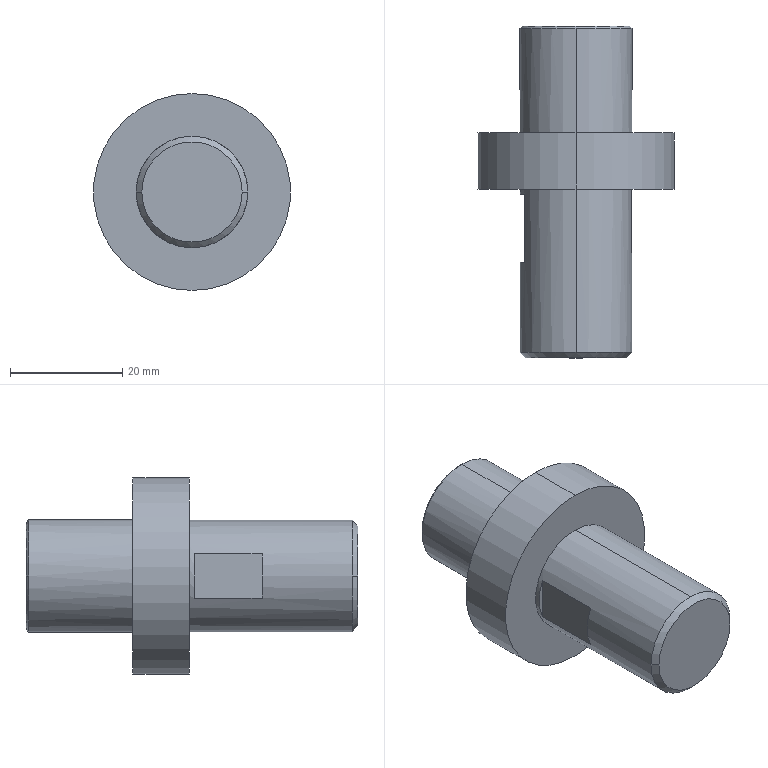Part | NX | 1 solid | 17 faces | box 35 x 59 x 35 mm | volume 24790 mm3 | plane 7 | cylinder 6 | cone 4 | commonest cylinder face diameters 19.857 x2 20 x2 35 x2
STEP:
#1=CARTESIAN_POINT('',(9.5,32.,0.));
#2=VERTEX_POINT('',#1);
#3=CARTESIAN_POINT('',(-9.5,32.,0.));
#4=VERTEX_POINT('',#3);
#5=CARTESIAN_POINT('',(0.,32.,0.));
#6=DIRECTION('',(0.,-1.,0.));
#7=DIRECTION('',(0.,0.,1.));
#8=AXIS2_PLACEMENT_3D('',#5,#6,#7);
#9=CIRCLE('',#8,9.5);
#10=EDGE_CURVE('',#2,#4,#9,.T.);
#11=ORIENTED_EDGE('',*,*,#10,.F.);
#12=CARTESIAN_POINT('',(0.,32.,0.));
#13=DIRECTION('',(0.,-1.,0.));
#14=DIRECTION('',(0.,0.,1.));
#15=AXIS2_PLACEMENT_3D('',#12,#13,#14);
#16=CIRCLE('',#15,9.5);
#17=EDGE_CURVE('',#4,#2,#16,.T.);
#18=ORIENTED_EDGE('',*,*,#17,.F.);
#19=EDGE_LOOP('',(#11,#18));
#20=FACE_BOUND('',#19,.T.);
#21=CARTESIAN_POINT('',(0.,32.,0.));
#22=DIRECTION('',(0.,1.,0.));
#23=DIRECTION('',(1.,0.,0.));
#24=AXIS2_PLACEMENT_3D('',#21,#22,#23);
#25=PLANE('',#24);
#26=ADVANCED_FACE('',(#20),#25,.T.);
#27=CARTESIAN_POINT('',(0.,31.5,-10.));
#28=VERTEX_POINT('',#27);
#29=CARTESIAN_POINT('',(10.,31.5,0.));
#30=VERTEX_POINT('',#29);
#31=CARTESIAN_POINT('',(0.,31.5,0.));
#32=DIRECTION('',(0.,-1.,0.));
#33=DIRECTION('',(0.,0.,1.));
#34=AXIS2_PLACEMENT_3D('',#31,#32,#33);
#35=CIRCLE('',#34,10.);
#36=EDGE_CURVE('',#28,#30,#35,.T.);
#37=ORIENTED_EDGE('',*,*,#36,.F.);
#38=CARTESIAN_POINT('',(-10.,31.5,0.));
#39=VERTEX_POINT('',#38);
#40=CARTESIAN_POINT('',(0.,31.5,0.));
#41=DIRECTION('',(0.,-1.,0.));
#42=DIRECTION('',(0.,0.,1.));
#43=AXIS2_PLACEMENT_3D('',#40,#41,#42);
#44=CIRCLE('',#43,10.);
#45=EDGE_CURVE('',#39,#28,#44,.T.);
#46=ORIENTED_EDGE('',*,*,#45,.F.);
#47=CARTESIAN_POINT('',(-9.75,31.75,0.));
#48=DIRECTION('',(-0.7071,-0.7071,0.));
#49=VECTOR('',#48,1000.);
#50=LINE('',#47,#49);
#51=EDGE_CURVE('',#39,#4,#50,.F.);
#52=ORIENTED_EDGE('',*,*,#51,.T.);
#53=ORIENTED_EDGE('',*,*,#17,.T.);
#54=CARTESIAN_POINT('',(9.75,31.75,0.));
#55=DIRECTION('',(0.7071,-0.7071,0.));
#56=VECTOR('',#55,1000.);
#57=LINE('',#54,#56);
#58=EDGE_CURVE('',#30,#2,#57,.F.);
#59=ORIENTED_EDGE('',*,*,#58,.F.);
#60=EDGE_LOOP('',(#37,#46,#52,#53,#59));
#61=FACE_BOUND('',#60,.T.);
#62=CARTESIAN_POINT('',(0.,31.75,0.));
#63=DIRECTION('',(0.,-1.,0.));
#64=DIRECTION('',(-1.,0.,0.));
#65=AXIS2_PLACEMENT_3D('',#62,#63,#64);
#66=CONICAL_SURFACE('',#65,9.75,0.7854);
#67=ADVANCED_FACE('',(#61),#66,.T.);
#68=CARTESIAN_POINT('',(0.,13.,10.));
#69=VERTEX_POINT('',#68);
#70=CARTESIAN_POINT('',(0.,13.,-10.));
#71=VERTEX_POINT('',#70);
#72=CARTESIAN_POINT('',(0.,13.,0.));
#73=DIRECTION('',(0.,1.,0.));
#74=DIRECTION('',(0.,0.,1.));
#75=AXIS2_PLACEMENT_3D('',#72,#73,#74);
#76=CIRCLE('',#75,10.);
#77=EDGE_CURVE('',#69,#71,#76,.T.);
#78=ORIENTED_EDGE('',*,*,#77,.T.);
#79=CARTESIAN_POINT('',(0.,-1.6,-10.));
#80=DIRECTION('',(0.,1.,0.));
#81=VECTOR('',#80,1000.);
#82=LINE('',#79,#81);
#83=EDGE_CURVE('',#71,#28,#82,.T.);
#84=ORIENTED_EDGE('',*,*,#83,.T.);
#85=ORIENTED_EDGE('',*,*,#36,.T.);
#86=CARTESIAN_POINT('',(0.,31.5,10.));
#87=VERTEX_POINT('',#86);
#88=CARTESIAN_POINT('',(0.,31.5,0.));
#89=DIRECTION('',(0.,-1.,0.));
#90=DIRECTION('',(0.,0.,1.));
#91=AXIS2_PLACEMENT_3D('',#88,#89,#90);
#92=CIRCLE('',#91,10.);
#93=EDGE_CURVE('',#30,#87,#92,.T.);
#94=ORIENTED_EDGE('',*,*,#93,.T.);
#95=CARTESIAN_POINT('',(0.,-1.6,10.));
#96=DIRECTION('',(0.,1.,0.));
#97=VECTOR('',#96,1000.);
#98=LINE('',#95,#97);
#99=EDGE_CURVE('',#69,#87,#98,.T.);
#100=ORIENTED_EDGE('',*,*,#99,.F.);
#101=EDGE_LOOP('',(#78,#84,#85,#94,#100));
#102=FACE_BOUND('',#101,.T.);
#103=CARTESIAN_POINT('',(0.,-1.6,0.));
#104=DIRECTION('',(0.,1.,0.));
#105=DIRECTION('',(0.,0.,1.));
#106=AXIS2_PLACEMENT_3D('',#103,#104,#105);
#107=CYLINDRICAL_SURFACE('',#106,10.);
#108=ADVANCED_FACE('',(#102),#107,.T.);
#109=CARTESIAN_POINT('',(0.,13.,-17.5));
#110=VERTEX_POINT('',#109);
#111=CARTESIAN_POINT('',(0.,13.,17.5));
#112=VERTEX_POINT('',#111);
#113=CARTESIAN_POINT('',(0.,13.,0.));
#114=DIRECTION('',(0.,-1.,0.));
#115=DIRECTION('',(0.,0.,1.));
#116=AXIS2_PLACEMENT_3D('',#113,#114,#115);
#117=CIRCLE('',#116,17.5);
#118=EDGE_CURVE('',#110,#112,#117,.T.);
#119=ORIENTED_EDGE('',*,*,#118,.F.);
#120=CARTESIAN_POINT('',(0.,13.,0.));
#121=DIRECTION('',(0.,-1.,0.));
#122=DIRECTION('',(0.,0.,1.));
#123=AXIS2_PLACEMENT_3D('',#120,#121,#122);
#124=CIRCLE('',#123,17.5);
#125=EDGE_CURVE('',#112,#110,#124,.T.);
#126=ORIENTED_EDGE('',*,*,#125,.F.);
#127=EDGE_LOOP('',(#119,#126));
#128=FACE_BOUND('',#127,.T.);
#129=ORIENTED_EDGE('',*,*,#77,.F.);
#130=CARTESIAN_POINT('',(0.,13.,0.));
#131=DIRECTION('',(0.,1.,0.));
#132=DIRECTION('',(0.,0.,1.));
#133=AXIS2_PLACEMENT_3D('',#130,#131,#132);
#134=CIRCLE('',#133,10.);
#135=EDGE_CURVE('',#71,#69,#134,.T.);
#136=ORIENTED_EDGE('',*,*,#135,.F.);
#137=EDGE_LOOP('',(#129,#136));
#138=FACE_BOUND('',#137,.T.);
#139=CARTESIAN_POINT('',(1.485,13.,-1.417));
#140=DIRECTION('',(0.,-1.,0.));
#141=DIRECTION('',(0.,0.,-1.));
#142=AXIS2_PLACEMENT_3D('',#139,#140,#141);
#143=PLANE('',#142);
#144=ADVANCED_FACE('',(#128,#138),#143,.F.);
#145=CARTESIAN_POINT('',(0.,3.,-17.5));
#146=VERTEX_POINT('',#145);
#147=CARTESIAN_POINT('',(0.,3.,17.5));
#148=VERTEX_POINT('',#147);
#149=CARTESIAN_POINT('',(0.,3.,0.));
#150=DIRECTION('',(0.,-1.,0.));
#151=DIRECTION('',(0.,0.,1.));
#152=AXIS2_PLACEMENT_3D('',#149,#150,#151);
#153=CIRCLE('',#152,17.5);
#154=EDGE_CURVE('',#146,#148,#153,.T.);
#155=ORIENTED_EDGE('',*,*,#154,.F.);
#156=CARTESIAN_POINT('',(0.,16.,-17.5));
#157=DIRECTION('',(0.,-1.,0.));
#158=VECTOR('',#157,1000.);
#159=LINE('',#156,#158);
#160=EDGE_CURVE('',#110,#146,#159,.T.);
#161=ORIENTED_EDGE('',*,*,#160,.F.);
#162=ORIENTED_EDGE('',*,*,#118,.T.);
#163=CARTESIAN_POINT('',(0.,16.,17.5));
#164=DIRECTION('',(0.,-1.,0.));
#165=VECTOR('',#164,1000.);
#166=LINE('',#163,#165);
#167=EDGE_CURVE('',#112,#148,#166,.T.);
#168=ORIENTED_EDGE('',*,*,#167,.T.);
#169=EDGE_LOOP('',(#155,#161,#162,#168));
#170=FACE_BOUND('',#169,.T.);
#171=CARTESIAN_POINT('',(0.,16.,0.));
#172=DIRECTION('',(0.,-1.,0.));
#173=DIRECTION('',(0.,0.,1.));
#174=AXIS2_PLACEMENT_3D('',#171,#172,#173);
#175=CYLINDRICAL_SURFACE('',#174,17.5);
#176=ADVANCED_FACE('',(#170),#175,.T.);
#177=ORIENTED_EDGE('',*,*,#154,.T.);
#178=CARTESIAN_POINT('',(0.,3.,0.));
#179=DIRECTION('',(0.,-1.,0.));
#180=DIRECTION('',(0.,0.,1.));
#181=AXIS2_PLACEMENT_3D('',#178,#179,#180);
#182=CIRCLE('',#181,17.5);
#183=EDGE_CURVE('',#148,#146,#182,.T.);
#184=ORIENTED_EDGE('',*,*,#183,.T.);
#185=EDGE_LOOP('',(#177,#184));
#186=FACE_BOUND('',#185,.T.);
#187=CARTESIAN_POINT('',(0.,3.,9.928));
#188=VERTEX_POINT('',#187);
#189=CARTESIAN_POINT('',(0.,3.,-9.928));
#190=VERTEX_POINT('',#189);
#191=CARTESIAN_POINT('',(0.,3.,0.));
#192=DIRECTION('',(0.,-1.,0.));
#193=DIRECTION('',(0.,0.,1.));
#194=AXIS2_PLACEMENT_3D('',#191,#192,#193);
#195=CIRCLE('',#194,9.928);
#196=EDGE_CURVE('',#188,#190,#195,.T.);
#197=ORIENTED_EDGE('',*,*,#196,.F.);
#198=CARTESIAN_POINT('',(0.,3.,0.));
#199=DIRECTION('',(0.,-1.,0.));
#200=DIRECTION('',(0.,0.,1.));
#201=AXIS2_PLACEMENT_3D('',#198,#199,#200);
#202=CIRCLE('',#201,9.928);
#203=EDGE_CURVE('',#190,#188,#202,.T.);
#204=ORIENTED_EDGE('',*,*,#203,.F.);
#205=EDGE_LOOP('',(#197,#204));
#206=FACE_BOUND('',#205,.T.);
#207=CARTESIAN_POINT('',(1.485,3.,-1.417));
#208=DIRECTION('',(0.,-1.,0.));
#209=DIRECTION('',(0.,0.,-1.));
#210=AXIS2_PLACEMENT_3D('',#207,#208,#209);
#211=PLANE('',#210);
#212=ADVANCED_FACE('',(#186,#206),#211,.T.);
#213=CARTESIAN_POINT('',(0.,-26.,-9.928));
#214=VERTEX_POINT('',#213);
#215=CARTESIAN_POINT('',(9.928,-26.,0.));
#216=VERTEX_POINT('',#215);
#217=CARTESIAN_POINT('',(0.,-26.,0.));
#218=DIRECTION('',(0.,-1.,0.));
#219=DIRECTION('',(-1.,0.,0.));
#220=AXIS2_PLACEMENT_3D('',#217,#218,#219);
#221=CIRCLE('',#220,9.928);
#222=EDGE_CURVE('',#214,#216,#221,.T.);
#223=ORIENTED_EDGE('',*,*,#222,.F.);
#224=CARTESIAN_POINT('',(0.,3.,-9.928));
#225=DIRECTION('',(0.,-1.,0.));
#226=VECTOR('',#225,1000.);
#227=LINE('',#224,#226);
#228=EDGE_CURVE('',#214,#190,#227,.F.);
#229=ORIENTED_EDGE('',*,*,#228,.T.);
#230=ORIENTED_EDGE('',*,*,#203,.T.);
#231=CARTESIAN_POINT('',(0.,-26.,9.928));
#232=VERTEX_POINT('',#231);
#233=CARTESIAN_POINT('',(0.,3.,9.928));
#234=DIRECTION('',(0.,-1.,0.));
#235=VECTOR('',#234,1000.);
#236=LINE('',#233,#235);
#237=EDGE_CURVE('',#232,#188,#236,.F.);
#238=ORIENTED_EDGE('',*,*,#237,.F.);
#239=CARTESIAN_POINT('',(0.,-26.,0.));
#240=DIRECTION('',(0.,-1.,0.));
#241=DIRECTION('',(-1.,0.,0.));
#242=AXIS2_PLACEMENT_3D('',#239,#240,#241);
#243=CIRCLE('',#242,9.928);
#244=EDGE_CURVE('',#216,#232,#243,.T.);
#245=ORIENTED_EDGE('',*,*,#244,.F.);
#246=EDGE_LOOP('',(#223,#229,#230,#238,#245));
#247=FACE_BOUND('',#246,.T.);
#248=CARTESIAN_POINT('',(0.,3.,0.));
#249=DIRECTION('',(0.,-1.,0.));
#250=DIRECTION('',(0.,0.,1.));
#251=AXIS2_PLACEMENT_3D('',#248,#249,#250);
#252=CYLINDRICAL_SURFACE('',#251,9.928);
#253=ADVANCED_FACE('',(#247),#252,.T.);
#254=CARTESIAN_POINT('',(8.928,-27.,0.));
#255=VERTEX_POINT('',#254);
#256=CARTESIAN_POINT('',(-8.928,-27.,0.));
#257=VERTEX_POINT('',#256);
#258=CARTESIAN_POINT('',(0.,-27.,0.));
#259=DIRECTION('',(0.,-1.,0.));
#260=DIRECTION('',(-1.,0.,0.));
#261=AXIS2_PLACEMENT_3D('',#258,#259,#260);
#262=CIRCLE('',#261,8.928);
#263=EDGE_CURVE('',#255,#257,#262,.T.);
#264=ORIENTED_EDGE('',*,*,#263,.T.);
#265=CARTESIAN_POINT('',(0.,-27.,0.));
#266=DIRECTION('',(0.,-1.,0.));
#267=DIRECTION('',(-1.,0.,0.));
#268=AXIS2_PLACEMENT_3D('',#265,#266,#267);
#269=CIRCLE('',#268,8.928);
#270=EDGE_CURVE('',#257,#255,#269,.T.);
#271=ORIENTED_EDGE('',*,*,#270,.T.);
#272=EDGE_LOOP('',(#264,#271));
#273=FACE_BOUND('',#272,.T.);
#274=CARTESIAN_POINT('',(-4.356,-27.,3.798));
#275=DIRECTION('',(0.,-1.,0.));
#276=DIRECTION('',(0.,0.,-1.));
#277=AXIS2_PLACEMENT_3D('',#274,#275,#276);
#278=PLANE('',#277);
#279=ADVANCED_FACE('',(#273),#278,.T.);
#280=CARTESIAN_POINT('',(-9.107,2.1,3.955));
#281=VERTEX_POINT('',#280);
#282=CARTESIAN_POINT('',(-9.107,2.1,-3.955));
#283=VERTEX_POINT('',#282);
#284=CARTESIAN_POINT('',(0.,2.1,0.));
#285=DIRECTION('',(0.,-1.,0.));
#286=DIRECTION('',(0.,0.,1.));
#287=AXIS2_PLACEMENT_3D('',#284,#285,#286);
#288=CIRCLE('',#287,9.928);
#289=EDGE_CURVE('',#281,#283,#288,.T.);
#290=ORIENTED_EDGE('',*,*,#289,.T.);
#291=CARTESIAN_POINT('',(-9.107,2.1,0.));
#292=DIRECTION('',(0.,0.,1.));
#293=VECTOR('',#292,1000.);
#294=LINE('',#291,#293);
#295=EDGE_CURVE('',#283,#281,#294,.T.);
#296=ORIENTED_EDGE('',*,*,#295,.T.);
#297=EDGE_LOOP('',(#290,#296));
#298=FACE_BOUND('',#297,.T.);
#299=CARTESIAN_POINT('',(-28.107,2.1,-21.002));
#300=DIRECTION('',(0.,1.,0.));
#301=DIRECTION('',(1.,0.,0.));
#302=AXIS2_PLACEMENT_3D('',#299,#300,#301);
#303=PLANE('',#302);
#304=ADVANCED_FACE('',(#298),#303,.F.);
#305=CARTESIAN_POINT('',(-9.107,-9.972,3.955));
#306=VERTEX_POINT('',#305);
#307=CARTESIAN_POINT('',(-9.107,-9.972,-3.955));
#308=VERTEX_POINT('',#307);
#309=CARTESIAN_POINT('',(0.,-9.972,0.));
#310=DIRECTION('',(0.,-1.,0.));
#311=DIRECTION('',(0.,0.,1.));
#312=AXIS2_PLACEMENT_3D('',#309,#310,#311);
#313=CIRCLE('',#312,9.928);
#314=EDGE_CURVE('',#306,#308,#313,.T.);
#315=ORIENTED_EDGE('',*,*,#314,.F.);
#316=CARTESIAN_POINT('',(-9.107,-9.972,0.));
#317=DIRECTION('',(0.,0.,1.));
#318=VECTOR('',#317,1000.);
#319=LINE('',#316,#318);
#320=EDGE_CURVE('',#308,#306,#319,.T.);
#321=ORIENTED_EDGE('',*,*,#320,.F.);
#322=EDGE_LOOP('',(#315,#321));
#323=FACE_BOUND('',#322,.T.);
#324=CARTESIAN_POINT('',(-5.107,-9.972,-21.002));
#325=DIRECTION('',(0.,-1.,0.));
#326=DIRECTION('',(0.,0.,-1.));
#327=AXIS2_PLACEMENT_3D('',#324,#325,#326);
#328=PLANE('',#327);
#329=ADVANCED_FACE('',(#323),#328,.F.);
#330=CARTESIAN_POINT('',(-9.107,3.,-3.955));
#331=DIRECTION('',(0.,-1.,0.));
#332=VECTOR('',#331,1000.);
#333=LINE('',#330,#332);
#334=EDGE_CURVE('',#308,#283,#333,.F.);
#335=ORIENTED_EDGE('',*,*,#334,.F.);
#336=ORIENTED_EDGE('',*,*,#320,.T.);
#337=CARTESIAN_POINT('',(-9.107,3.,3.955));
#338=DIRECTION('',(0.,-1.,0.));
#339=VECTOR('',#338,1000.);
#340=LINE('',#337,#339);
#341=EDGE_CURVE('',#306,#281,#340,.F.);
#342=ORIENTED_EDGE('',*,*,#341,.T.);
#343=ORIENTED_EDGE('',*,*,#295,.F.);
#344=EDGE_LOOP('',(#335,#336,#342,#343));
#345=FACE_BOUND('',#344,.T.);
#346=CARTESIAN_POINT('',(-9.107,2.028,-21.002));
#347=DIRECTION('',(1.,0.,0.));
#348=DIRECTION('',(0.,1.,0.));
#349=AXIS2_PLACEMENT_3D('',#346,#347,#348);
#350=PLANE('',#349);
#351=ADVANCED_FACE('',(#345),#350,.F.);
#352=ORIENTED_EDGE('',*,*,#222,.T.);
#353=CARTESIAN_POINT('',(8.928,-27.,0.));
#354=DIRECTION('',(0.7071,0.7071,0.));
#355=VECTOR('',#354,1000.);
#356=LINE('',#353,#355);
#357=EDGE_CURVE('',#255,#216,#356,.T.);
#358=ORIENTED_EDGE('',*,*,#357,.F.);
#359=ORIENTED_EDGE('',*,*,#270,.F.);
#360=CARTESIAN_POINT('',(-9.928,-26.,0.));
#361=VERTEX_POINT('',#360);
#362=CARTESIAN_POINT('',(-8.928,-27.,0.));
#363=DIRECTION('',(-0.7071,0.7071,0.));
#364=VECTOR('',#363,1000.);
#365=LINE('',#362,#364);
#366=EDGE_CURVE('',#257,#361,#365,.T.);
#367=ORIENTED_EDGE('',*,*,#366,.T.);
#368=CARTESIAN_POINT('',(0.,-26.,0.));
#369=DIRECTION('',(0.,-1.,0.));
#370=DIRECTION('',(-1.,0.,0.));
#371=AXIS2_PLACEMENT_3D('',#368,#369,#370);
#372=CIRCLE('',#371,9.928);
#373=EDGE_CURVE('',#361,#214,#372,.T.);
#374=ORIENTED_EDGE('',*,*,#373,.T.);
#375=EDGE_LOOP('',(#352,#358,#359,#367,#374));
#376=FACE_BOUND('',#375,.T.);
#377=CARTESIAN_POINT('',(0.,-27.,0.));
#378=DIRECTION('',(0.,1.,0.));
#379=DIRECTION('',(1.,0.,0.));
#380=AXIS2_PLACEMENT_3D('',#377,#378,#379);
#381=CONICAL_SURFACE('',#380,8.928,0.7854);
#382=ADVANCED_FACE('',(#376),#381,.T.);
#383=ORIENTED_EDGE('',*,*,#99,.T.);
#384=CARTESIAN_POINT('',(0.,31.5,0.));
#385=DIRECTION('',(0.,-1.,0.));
#386=DIRECTION('',(0.,0.,1.));
#387=AXIS2_PLACEMENT_3D('',#384,#385,#386);
#388=CIRCLE('',#387,10.);
#389=EDGE_CURVE('',#87,#39,#388,.T.);
#390=ORIENTED_EDGE('',*,*,#389,.T.);
#391=ORIENTED_EDGE('',*,*,#45,.T.);
#392=ORIENTED_EDGE('',*,*,#83,.F.);
#393=ORIENTED_EDGE('',*,*,#135,.T.);
#394=EDGE_LOOP('',(#383,#390,#391,#392,#393));
#395=FACE_BOUND('',#394,.T.);
#396=CARTESIAN_POINT('',(0.,-1.6,0.));
#397=DIRECTION('',(0.,1.,0.));
#398=DIRECTION('',(0.,0.,1.));
#399=AXIS2_PLACEMENT_3D('',#396,#397,#398);
#400=CYLINDRICAL_SURFACE('',#399,10.);
#401=ADVANCED_FACE('',(#395),#400,.T.);
#402=ORIENTED_EDGE('',*,*,#10,.T.);
#403=ORIENTED_EDGE('',*,*,#51,.F.);
#404=ORIENTED_EDGE('',*,*,#389,.F.);
#405=ORIENTED_EDGE('',*,*,#93,.F.);
#406=ORIENTED_EDGE('',*,*,#58,.T.);
#407=EDGE_LOOP('',(#402,#403,#404,#405,#406));
#408=FACE_BOUND('',#407,.T.);
#409=CARTESIAN_POINT('',(0.,31.75,0.));
#410=DIRECTION('',(0.,-1.,0.));
#411=DIRECTION('',(-1.,0.,0.));
#412=AXIS2_PLACEMENT_3D('',#409,#410,#411);
#413=CONICAL_SURFACE('',#412,9.75,0.7854);
#414=ADVANCED_FACE('',(#408),#413,.T.);
#415=ORIENTED_EDGE('',*,*,#263,.F.);
#416=ORIENTED_EDGE('',*,*,#357,.T.);
#417=ORIENTED_EDGE('',*,*,#244,.T.);
#418=CARTESIAN_POINT('',(0.,-26.,0.));
#419=DIRECTION('',(0.,-1.,0.));
#420=DIRECTION('',(-1.,0.,0.));
#421=AXIS2_PLACEMENT_3D('',#418,#419,#420);
#422=CIRCLE('',#421,9.928);
#423=EDGE_CURVE('',#232,#361,#422,.T.);
#424=ORIENTED_EDGE('',*,*,#423,.T.);
#425=ORIENTED_EDGE('',*,*,#366,.F.);
#426=EDGE_LOOP('',(#415,#416,#417,#424,#425));
#427=FACE_BOUND('',#426,.T.);
#428=CARTESIAN_POINT('',(0.,-27.,0.));
#429=DIRECTION('',(0.,1.,0.));
#430=DIRECTION('',(1.,0.,0.));
#431=AXIS2_PLACEMENT_3D('',#428,#429,#430);
#432=CONICAL_SURFACE('',#431,8.928,0.7854);
#433=ADVANCED_FACE('',(#427),#432,.T.);
#434=ORIENTED_EDGE('',*,*,#196,.T.);
#435=ORIENTED_EDGE('',*,*,#228,.F.);
#436=ORIENTED_EDGE('',*,*,#373,.F.);
#437=ORIENTED_EDGE('',*,*,#423,.F.);
#438=ORIENTED_EDGE('',*,*,#237,.T.);
#439=EDGE_LOOP('',(#434,#435,#436,#437,#438));
#440=FACE_BOUND('',#439,.T.);
#441=ORIENTED_EDGE('',*,*,#334,.T.);
#442=ORIENTED_EDGE('',*,*,#289,.F.);
#443=ORIENTED_EDGE('',*,*,#341,.F.);
#444=ORIENTED_EDGE('',*,*,#314,.T.);
#445=EDGE_LOOP('',(#441,#442,#443,#444));
#446=FACE_BOUND('',#445,.T.);
#447=CARTESIAN_POINT('',(0.,3.,0.));
#448=DIRECTION('',(0.,-1.,0.));
#449=DIRECTION('',(0.,0.,1.));
#450=AXIS2_PLACEMENT_3D('',#447,#448,#449);
#451=CYLINDRICAL_SURFACE('',#450,9.928);
#452=ADVANCED_FACE('',(#440,#446),#451,.T.);
#453=ORIENTED_EDGE('',*,*,#167,.F.);
#454=ORIENTED_EDGE('',*,*,#125,.T.);
#455=ORIENTED_EDGE('',*,*,#160,.T.);
#456=ORIENTED_EDGE('',*,*,#183,.F.);
#457=EDGE_LOOP('',(#453,#454,#455,#456));
#458=FACE_BOUND('',#457,.T.);
#459=CARTESIAN_POINT('',(0.,16.,0.));
#460=DIRECTION('',(0.,-1.,0.));
#461=DIRECTION('',(0.,0.,1.));
#462=AXIS2_PLACEMENT_3D('',#459,#460,#461);
#463=CYLINDRICAL_SURFACE('',#462,17.5);
#464=ADVANCED_FACE('',(#458),#463,.T.);
#465=CLOSED_SHELL('',(#26,#67,#108,#144,#176,#212,#253,#279,#304,#329,#351,#382,#401,#414,#433,#452,#464));
#466=MANIFOLD_SOLID_BREP('',#465);
#467=(LENGTH_UNIT()NAMED_UNIT(*)SI_UNIT(.MILLI.,.METRE.));
#468=UNCERTAINTY_MEASURE_WITH_UNIT(LENGTH_MEASURE(0.00001),#467,'','');
#469=(NAMED_UNIT(*)PLANE_ANGLE_UNIT()SI_UNIT($,.RADIAN.));
#470=(NAMED_UNIT(*)SI_UNIT($,.STERADIAN.)SOLID_ANGLE_UNIT());
#471=(GEOMETRIC_REPRESENTATION_CONTEXT(3)GLOBAL_UNCERTAINTY_ASSIGNED_CONTEXT((#468))GLOBAL_UNIT_ASSIGNED_CONTEXT((#467,#469,#470))REPRESENTATION_CONTEXT('',''));
#472=ADVANCED_BREP_SHAPE_REPRESENTATION('',(#466),#471);